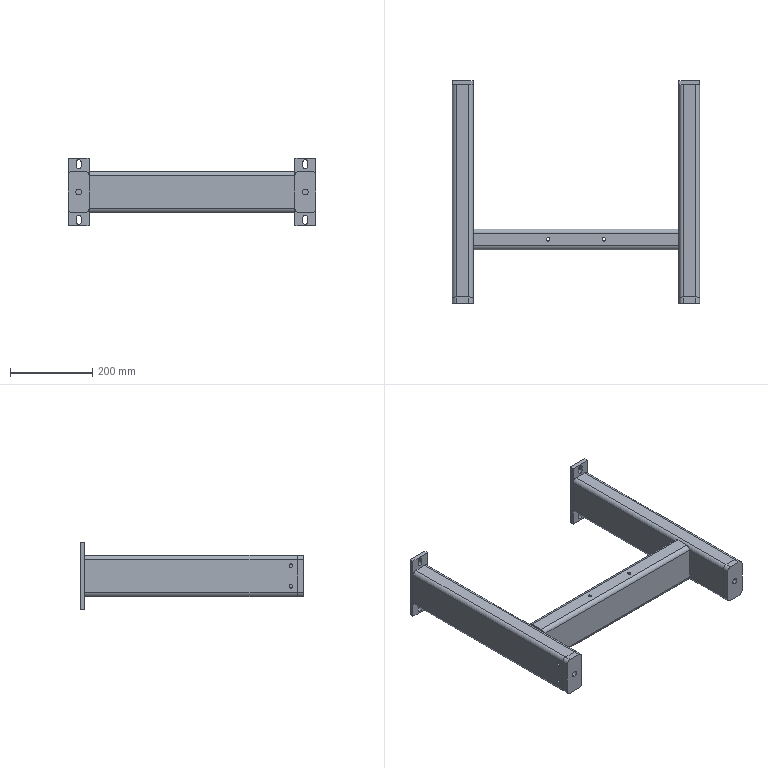Part | STEP file | PN_0054_frame_default_machined_ | 7 solids | 126 faces | box 600 x 540 x 165 mm | volume 2339711 mm3 | cylinder 64 | plane 62 | commonest cylinder face diameters 20 x20 8.5 x16 10 x12 12 x12 14 x4